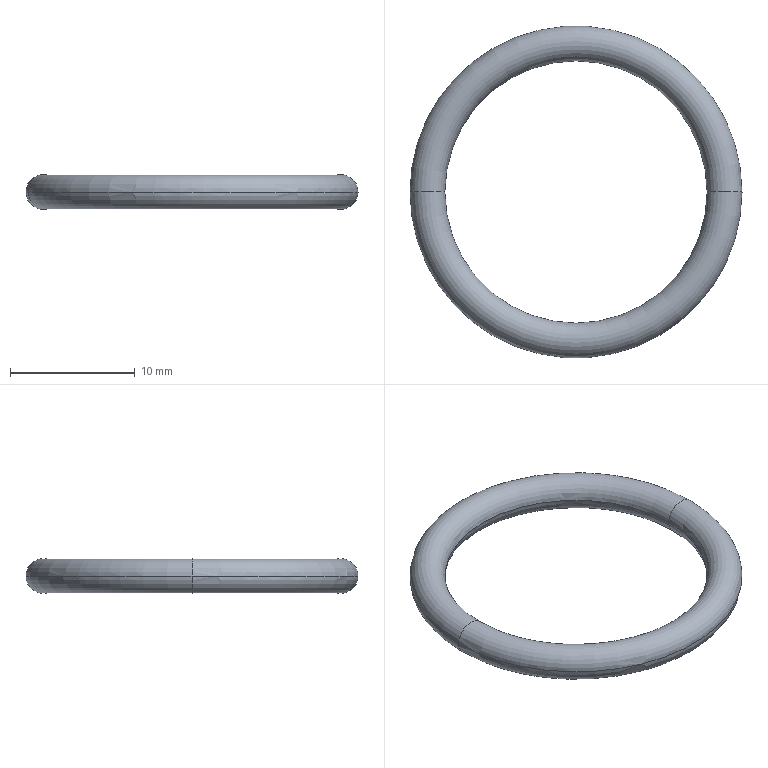Part | STEP file | ZXW722-L-40 | 1 solid | 4 faces | box 26.66 x 26.66 x 2.8 mm | volume 461.558 mm3 | torus 4
STEP:
#1=CARTESIAN_POINT('',(0.,0.,0.));
#2=DIRECTION('',(0.,0.,1.));
#3=DIRECTION('',(1.,0.,0.));
#4=AXIS2_PLACEMENT_3D('',#1,#2,#3);
#5=CARTESIAN_POINT('',(-10.53,0.,1.32));
#6=VERTEX_POINT('',#5);
#7=CARTESIAN_POINT('',(-13.33,0.,1.32));
#8=VERTEX_POINT('',#7);
#9=CARTESIAN_POINT('',(-11.93,0.,1.32));
#10=DIRECTION('',(0.,-1.,0.));
#11=DIRECTION('',(1.,0.,0.));
#12=AXIS2_PLACEMENT_3D('',#9,#10,#11);
#13=CIRCLE('',#12,1.4);
#14=EDGE_CURVE('',#6,#8,#13,.T.);
#15=ORIENTED_EDGE('',*,*,#14,.T.);
#16=CARTESIAN_POINT('',(13.33,0.,1.32));
#17=VERTEX_POINT('',#16);
#18=CARTESIAN_POINT('',(0.,0.,1.32));
#19=DIRECTION('',(0.,0.,-1.));
#20=DIRECTION('',(-1.,0.,0.));
#21=AXIS2_PLACEMENT_3D('',#18,#19,#20);
#22=CIRCLE('',#21,13.33);
#23=EDGE_CURVE('',#8,#17,#22,.T.);
#24=ORIENTED_EDGE('',*,*,#23,.T.);
#25=CARTESIAN_POINT('',(10.53,0.,1.32));
#26=VERTEX_POINT('',#25);
#27=CARTESIAN_POINT('',(11.93,0.,1.32));
#28=DIRECTION('',(0.,1.,0.));
#29=DIRECTION('',(-1.,0.,0.));
#30=AXIS2_PLACEMENT_3D('',#27,#28,#29);
#31=CIRCLE('',#30,1.4);
#32=EDGE_CURVE('',#26,#17,#31,.T.);
#33=ORIENTED_EDGE('',*,*,#32,.F.);
#34=CARTESIAN_POINT('',(0.,0.,1.32));
#35=DIRECTION('',(0.,0.,-1.));
#36=DIRECTION('',(-1.,0.,0.));
#37=AXIS2_PLACEMENT_3D('',#34,#35,#36);
#38=CIRCLE('',#37,10.53);
#39=EDGE_CURVE('',#6,#26,#38,.T.);
#40=ORIENTED_EDGE('',*,*,#39,.F.);
#41=EDGE_LOOP('',(#15,#24,#33,#40));
#42=FACE_OUTER_BOUND('',#41,.F.);
#43=CARTESIAN_POINT('',(0.,0.,1.32));
#44=DIRECTION('',(0.,0.,-1.));
#45=DIRECTION('',(-1.,0.,0.));
#46=AXIS2_PLACEMENT_3D('',#43,#44,#45);
#47=TOROIDAL_SURFACE('',#46,11.93,1.4);
#48=ADVANCED_FACE('',(#42),#47,.T.);
#49=ORIENTED_EDGE('',*,*,#14,.F.);
#50=CARTESIAN_POINT('',(0.,0.,1.32));
#51=DIRECTION('',(0.,0.,1.));
#52=DIRECTION('',(-1.,0.,0.));
#53=AXIS2_PLACEMENT_3D('',#50,#51,#52);
#54=CIRCLE('',#53,10.53);
#55=EDGE_CURVE('',#6,#26,#54,.T.);
#56=ORIENTED_EDGE('',*,*,#55,.T.);
#57=ORIENTED_EDGE('',*,*,#32,.T.);
#58=CARTESIAN_POINT('',(0.,0.,1.32));
#59=DIRECTION('',(0.,0.,1.));
#60=DIRECTION('',(-1.,0.,0.));
#61=AXIS2_PLACEMENT_3D('',#58,#59,#60);
#62=CIRCLE('',#61,13.33);
#63=EDGE_CURVE('',#8,#17,#62,.T.);
#64=ORIENTED_EDGE('',*,*,#63,.F.);
#65=EDGE_LOOP('',(#49,#56,#57,#64));
#66=FACE_OUTER_BOUND('',#65,.F.);
#67=CARTESIAN_POINT('',(0.,0.,1.32));
#68=DIRECTION('',(0.,0.,-1.));
#69=DIRECTION('',(-1.,0.,0.));
#70=AXIS2_PLACEMENT_3D('',#67,#68,#69);
#71=TOROIDAL_SURFACE('',#70,11.93,1.4);
#72=ADVANCED_FACE('',(#66),#71,.T.);
#73=CARTESIAN_POINT('',(-11.93,0.,1.32));
#74=DIRECTION('',(0.,-1.,0.));
#75=DIRECTION('',(-1.,0.,0.));
#76=AXIS2_PLACEMENT_3D('',#73,#74,#75);
#77=CIRCLE('',#76,1.4);
#78=EDGE_CURVE('',#8,#6,#77,.T.);
#79=ORIENTED_EDGE('',*,*,#78,.F.);
#80=ORIENTED_EDGE('',*,*,#63,.T.);
#81=CARTESIAN_POINT('',(11.93,0.,1.32));
#82=DIRECTION('',(0.,1.,0.));
#83=DIRECTION('',(1.,0.,0.));
#84=AXIS2_PLACEMENT_3D('',#81,#82,#83);
#85=CIRCLE('',#84,1.4);
#86=EDGE_CURVE('',#17,#26,#85,.T.);
#87=ORIENTED_EDGE('',*,*,#86,.T.);
#88=ORIENTED_EDGE('',*,*,#55,.F.);
#89=EDGE_LOOP('',(#79,#80,#87,#88));
#90=FACE_OUTER_BOUND('',#89,.F.);
#91=CARTESIAN_POINT('',(0.,0.,1.32));
#92=DIRECTION('',(0.,0.,-1.));
#93=DIRECTION('',(-1.,0.,0.));
#94=AXIS2_PLACEMENT_3D('',#91,#92,#93);
#95=TOROIDAL_SURFACE('',#94,11.93,1.4);
#96=ADVANCED_FACE('',(#90),#95,.T.);
#97=ORIENTED_EDGE('',*,*,#78,.T.);
#98=ORIENTED_EDGE('',*,*,#39,.T.);
#99=ORIENTED_EDGE('',*,*,#86,.F.);
#100=ORIENTED_EDGE('',*,*,#23,.F.);
#101=EDGE_LOOP('',(#97,#98,#99,#100));
#102=FACE_OUTER_BOUND('',#101,.F.);
#103=CARTESIAN_POINT('',(0.,0.,1.32));
#104=DIRECTION('',(0.,0.,-1.));
#105=DIRECTION('',(-1.,0.,0.));
#106=AXIS2_PLACEMENT_3D('',#103,#104,#105);
#107=TOROIDAL_SURFACE('',#106,11.93,1.4);
#108=ADVANCED_FACE('',(#102),#107,.T.);
#109=CLOSED_SHELL('',(#48,#72,#96,#108));
#110=MANIFOLD_SOLID_BREP('',#109);
#111=(LENGTH_UNIT()NAMED_UNIT(*)SI_UNIT(.MILLI.,.METRE.));
#112=UNCERTAINTY_MEASURE_WITH_UNIT(LENGTH_MEASURE(0.003781),#111,'','');
#113=(NAMED_UNIT(*)PLANE_ANGLE_UNIT()SI_UNIT($,.RADIAN.));
#114=PLANE_ANGLE_MEASURE_WITH_UNIT(PLANE_ANGLE_MEASURE(0.01745),#113);
#115=(CONVERSION_BASED_UNIT('DEGREE',#114)NAMED_UNIT(*)PLANE_ANGLE_UNIT());
#116=(NAMED_UNIT(*)SI_UNIT($,.STERADIAN.)SOLID_ANGLE_UNIT());
#117=(GEOMETRIC_REPRESENTATION_CONTEXT(3)GLOBAL_UNCERTAINTY_ASSIGNED_CONTEXT((#112))GLOBAL_UNIT_ASSIGNED_CONTEXT((#111,#115,#116))REPRESENTATION_CONTEXT('',''));
#118=ADVANCED_BREP_SHAPE_REPRESENTATION('',(#4,#110),#117);